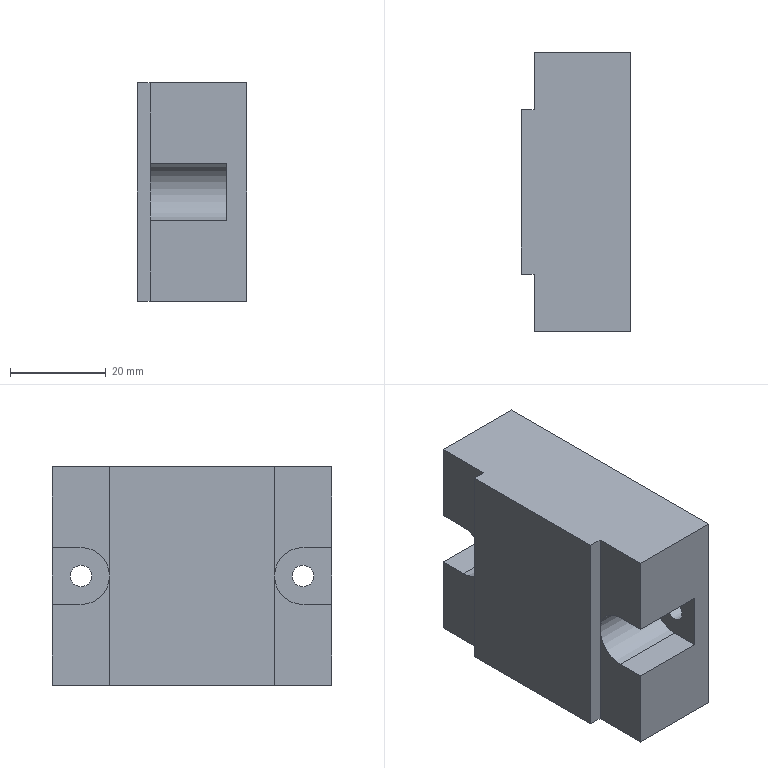Part | NX | features 5003_025_GSR-10L-D32Z 2 | 1 solid | 20 faces | box 22.9 x 58.4 x 45.7 mm | volume 53958 mm3 | plane 16 | cylinder 4 | commonest cylinder face diameters 4.5 x2 11.9 x2
STEP:
#1=CARTESIAN_POINT('',(-263.675,-496.,-115.8));
#2=VERTEX_POINT('',#1);
#3=CARTESIAN_POINT('',(-263.675,-502.,-115.8));
#4=VERTEX_POINT('',#3);
#5=CARTESIAN_POINT('',(-263.675,-502.,-115.8));
#6=DIRECTION('',(0.,-1.,0.));
#7=VECTOR('',#6,1000.);
#8=LINE('',#5,#7);
#9=EDGE_CURVE('',#2,#4,#8,.T.);
#10=ORIENTED_EDGE('',*,*,#9,.F.);
#11=CARTESIAN_POINT('',(-263.675,-496.,-132.7));
#12=VERTEX_POINT('',#11);
#13=CARTESIAN_POINT('',(-263.675,-496.,-87.));
#14=DIRECTION('',(0.,0.,-1.));
#15=VECTOR('',#14,1000.);
#16=LINE('',#13,#15);
#17=EDGE_CURVE('',#2,#12,#16,.T.);
#18=ORIENTED_EDGE('',*,*,#17,.T.);
#19=CARTESIAN_POINT('',(-263.675,-508.,-132.7));
#20=VERTEX_POINT('',#19);
#21=CARTESIAN_POINT('',(-263.675,-496.,-132.7));
#22=DIRECTION('',(0.,-1.,0.));
#23=VECTOR('',#22,1000.);
#24=LINE('',#21,#23);
#25=EDGE_CURVE('',#12,#20,#24,.T.);
#26=ORIENTED_EDGE('',*,*,#25,.T.);
#27=CARTESIAN_POINT('',(-263.675,-508.,-87.));
#28=VERTEX_POINT('',#27);
#29=CARTESIAN_POINT('',(-263.675,-508.,-87.));
#30=DIRECTION('',(0.,0.,-1.));
#31=VECTOR('',#30,1000.);
#32=LINE('',#29,#31);
#33=EDGE_CURVE('',#28,#20,#32,.T.);
#34=ORIENTED_EDGE('',*,*,#33,.F.);
#35=CARTESIAN_POINT('',(-263.675,-496.,-87.));
#36=VERTEX_POINT('',#35);
#37=CARTESIAN_POINT('',(-263.675,-496.,-87.));
#38=DIRECTION('',(0.,1.,0.));
#39=VECTOR('',#38,1000.);
#40=LINE('',#37,#39);
#41=EDGE_CURVE('',#28,#36,#40,.T.);
#42=ORIENTED_EDGE('',*,*,#41,.T.);
#43=CARTESIAN_POINT('',(-263.675,-496.,-103.9));
#44=VERTEX_POINT('',#43);
#45=CARTESIAN_POINT('',(-263.675,-496.,-87.));
#46=DIRECTION('',(0.,0.,-1.));
#47=VECTOR('',#46,1000.);
#48=LINE('',#45,#47);
#49=EDGE_CURVE('',#36,#44,#48,.T.);
#50=ORIENTED_EDGE('',*,*,#49,.T.);
#51=CARTESIAN_POINT('',(-263.675,-502.,-103.9));
#52=VERTEX_POINT('',#51);
#53=CARTESIAN_POINT('',(-263.675,-502.,-103.9));
#54=DIRECTION('',(0.,1.,0.));
#55=VECTOR('',#54,1000.);
#56=LINE('',#53,#55);
#57=EDGE_CURVE('',#52,#44,#56,.T.);
#58=ORIENTED_EDGE('',*,*,#57,.F.);
#59=CARTESIAN_POINT('',(-263.675,-502.,-109.85));
#60=DIRECTION('',(-1.,0.,0.));
#61=DIRECTION('',(0.,0.,-1.));
#62=AXIS2_PLACEMENT_3D('',#59,#60,#61);
#63=CIRCLE('',#62,5.95);
#64=EDGE_CURVE('',#4,#52,#63,.T.);
#65=ORIENTED_EDGE('',*,*,#64,.F.);
#66=EDGE_LOOP('',(#10,#18,#26,#34,#42,#50,#58,#65));
#67=FACE_BOUND('',#66,.T.);
#68=CARTESIAN_POINT('',(-263.675,-496.,-87.));
#69=DIRECTION('',(-1.,0.,0.));
#70=DIRECTION('',(0.,0.,-1.));
#71=AXIS2_PLACEMENT_3D('',#68,#69,#70);
#72=PLANE('',#71);
#73=ADVANCED_FACE('',(#67),#72,.T.);
#74=ORIENTED_EDGE('',*,*,#17,.F.);
#75=CARTESIAN_POINT('',(-247.675,-496.,-115.8));
#76=VERTEX_POINT('',#75);
#77=CARTESIAN_POINT('',(-247.675,-496.,-115.8));
#78=DIRECTION('',(-1.,0.,0.));
#79=VECTOR('',#78,1000.);
#80=LINE('',#77,#79);
#81=EDGE_CURVE('',#76,#2,#80,.T.);
#82=ORIENTED_EDGE('',*,*,#81,.F.);
#83=CARTESIAN_POINT('',(-247.675,-496.,-103.9));
#84=VERTEX_POINT('',#83);
#85=CARTESIAN_POINT('',(-247.675,-496.,-115.8));
#86=DIRECTION('',(0.,0.,-1.));
#87=VECTOR('',#86,1000.);
#88=LINE('',#85,#87);
#89=EDGE_CURVE('',#84,#76,#88,.T.);
#90=ORIENTED_EDGE('',*,*,#89,.F.);
#91=CARTESIAN_POINT('',(-247.675,-496.,-103.9));
#92=DIRECTION('',(-1.,0.,0.));
#93=VECTOR('',#92,1000.);
#94=LINE('',#91,#93);
#95=EDGE_CURVE('',#84,#44,#94,.T.);
#96=ORIENTED_EDGE('',*,*,#95,.T.);
#97=ORIENTED_EDGE('',*,*,#49,.F.);
#98=CARTESIAN_POINT('',(-243.475,-496.,-87.));
#99=VERTEX_POINT('',#98);
#100=CARTESIAN_POINT('',(-263.675,-496.,-87.));
#101=DIRECTION('',(1.,0.,0.));
#102=VECTOR('',#101,1000.);
#103=LINE('',#100,#102);
#104=EDGE_CURVE('',#36,#99,#103,.T.);
#105=ORIENTED_EDGE('',*,*,#104,.T.);
#106=CARTESIAN_POINT('',(-243.475,-496.,-132.7));
#107=VERTEX_POINT('',#106);
#108=CARTESIAN_POINT('',(-243.475,-496.,-87.));
#109=DIRECTION('',(0.,0.,-1.));
#110=VECTOR('',#109,1000.);
#111=LINE('',#108,#110);
#112=EDGE_CURVE('',#99,#107,#111,.T.);
#113=ORIENTED_EDGE('',*,*,#112,.T.);
#114=CARTESIAN_POINT('',(-263.675,-496.,-132.7));
#115=DIRECTION('',(1.,0.,0.));
#116=VECTOR('',#115,1000.);
#117=LINE('',#114,#116);
#118=EDGE_CURVE('',#12,#107,#117,.T.);
#119=ORIENTED_EDGE('',*,*,#118,.F.);
#120=EDGE_LOOP('',(#74,#82,#90,#96,#97,#105,#113,#119));
#121=FACE_BOUND('',#120,.T.);
#122=CARTESIAN_POINT('',(-263.675,-496.,-87.));
#123=DIRECTION('',(0.,-1.,0.));
#124=DIRECTION('',(0.,0.,1.));
#125=AXIS2_PLACEMENT_3D('',#122,#123,#124);
#126=PLANE('',#125);
#127=ADVANCED_FACE('',(#121),#126,.F.);
#128=CARTESIAN_POINT('',(-243.475,-554.4,-132.7));
#129=VERTEX_POINT('',#128);
#130=CARTESIAN_POINT('',(-243.475,-496.,-132.7));
#131=DIRECTION('',(0.,-1.,0.));
#132=VECTOR('',#131,1000.);
#133=LINE('',#130,#132);
#134=EDGE_CURVE('',#107,#129,#133,.T.);
#135=ORIENTED_EDGE('',*,*,#134,.T.);
#136=CARTESIAN_POINT('',(-263.675,-554.4,-132.7));
#137=VERTEX_POINT('',#136);
#138=CARTESIAN_POINT('',(-263.675,-554.4,-132.7));
#139=DIRECTION('',(1.,0.,0.));
#140=VECTOR('',#139,1000.);
#141=LINE('',#138,#140);
#142=EDGE_CURVE('',#137,#129,#141,.T.);
#143=ORIENTED_EDGE('',*,*,#142,.F.);
#144=CARTESIAN_POINT('',(-263.675,-542.4,-132.7));
#145=VERTEX_POINT('',#144);
#146=CARTESIAN_POINT('',(-263.675,-496.,-132.7));
#147=DIRECTION('',(0.,-1.,0.));
#148=VECTOR('',#147,1000.);
#149=LINE('',#146,#148);
#150=EDGE_CURVE('',#145,#137,#149,.T.);
#151=ORIENTED_EDGE('',*,*,#150,.F.);
#152=CARTESIAN_POINT('',(-266.375,-542.4,-132.7));
#153=VERTEX_POINT('',#152);
#154=CARTESIAN_POINT('',(-266.375,-542.4,-132.7));
#155=DIRECTION('',(1.,0.,0.));
#156=VECTOR('',#155,1000.);
#157=LINE('',#154,#156);
#158=EDGE_CURVE('',#153,#145,#157,.T.);
#159=ORIENTED_EDGE('',*,*,#158,.F.);
#160=CARTESIAN_POINT('',(-266.375,-508.,-132.7));
#161=VERTEX_POINT('',#160);
#162=CARTESIAN_POINT('',(-266.375,-508.,-132.7));
#163=DIRECTION('',(0.,-1.,0.));
#164=VECTOR('',#163,1000.);
#165=LINE('',#162,#164);
#166=EDGE_CURVE('',#161,#153,#165,.T.);
#167=ORIENTED_EDGE('',*,*,#166,.F.);
#168=CARTESIAN_POINT('',(-266.375,-508.,-132.7));
#169=DIRECTION('',(1.,0.,0.));
#170=VECTOR('',#169,1000.);
#171=LINE('',#168,#170);
#172=EDGE_CURVE('',#161,#20,#171,.T.);
#173=ORIENTED_EDGE('',*,*,#172,.T.);
#174=ORIENTED_EDGE('',*,*,#25,.F.);
#175=ORIENTED_EDGE('',*,*,#118,.T.);
#176=EDGE_LOOP('',(#135,#143,#151,#159,#167,#173,#174,#175));
#177=FACE_BOUND('',#176,.T.);
#178=CARTESIAN_POINT('',(-263.675,-496.,-132.7));
#179=DIRECTION('',(0.,0.,1.));
#180=DIRECTION('',(0.,1.,0.));
#181=AXIS2_PLACEMENT_3D('',#178,#179,#180);
#182=PLANE('',#181);
#183=ADVANCED_FACE('',(#177),#182,.F.);
#184=CARTESIAN_POINT('',(-263.675,-554.4,-103.9));
#185=VERTEX_POINT('',#184);
#186=CARTESIAN_POINT('',(-263.675,-554.4,-87.));
#187=VERTEX_POINT('',#186);
#188=CARTESIAN_POINT('',(-263.675,-554.4,-87.));
#189=DIRECTION('',(0.,0.,1.));
#190=VECTOR('',#189,1000.);
#191=LINE('',#188,#190);
#192=EDGE_CURVE('',#185,#187,#191,.T.);
#193=ORIENTED_EDGE('',*,*,#192,.F.);
#194=CARTESIAN_POINT('',(-247.675,-554.4,-103.9));
#195=VERTEX_POINT('',#194);
#196=CARTESIAN_POINT('',(-247.675,-554.4,-103.9));
#197=DIRECTION('',(-1.,0.,0.));
#198=VECTOR('',#197,1000.);
#199=LINE('',#196,#198);
#200=EDGE_CURVE('',#195,#185,#199,.T.);
#201=ORIENTED_EDGE('',*,*,#200,.F.);
#202=CARTESIAN_POINT('',(-247.675,-554.4,-115.8));
#203=VERTEX_POINT('',#202);
#204=CARTESIAN_POINT('',(-247.675,-554.4,-115.8));
#205=DIRECTION('',(0.,0.,1.));
#206=VECTOR('',#205,1000.);
#207=LINE('',#204,#206);
#208=EDGE_CURVE('',#203,#195,#207,.T.);
#209=ORIENTED_EDGE('',*,*,#208,.F.);
#210=CARTESIAN_POINT('',(-263.675,-554.4,-115.8));
#211=VERTEX_POINT('',#210);
#212=CARTESIAN_POINT('',(-247.675,-554.4,-115.8));
#213=DIRECTION('',(-1.,0.,0.));
#214=VECTOR('',#213,1000.);
#215=LINE('',#212,#214);
#216=EDGE_CURVE('',#203,#211,#215,.T.);
#217=ORIENTED_EDGE('',*,*,#216,.T.);
#218=CARTESIAN_POINT('',(-263.675,-554.4,-87.));
#219=DIRECTION('',(0.,0.,1.));
#220=VECTOR('',#219,1000.);
#221=LINE('',#218,#220);
#222=EDGE_CURVE('',#137,#211,#221,.T.);
#223=ORIENTED_EDGE('',*,*,#222,.F.);
#224=ORIENTED_EDGE('',*,*,#142,.T.);
#225=CARTESIAN_POINT('',(-243.475,-554.4,-87.));
#226=VERTEX_POINT('',#225);
#227=CARTESIAN_POINT('',(-243.475,-554.4,-87.));
#228=DIRECTION('',(0.,0.,1.));
#229=VECTOR('',#228,1000.);
#230=LINE('',#227,#229);
#231=EDGE_CURVE('',#129,#226,#230,.T.);
#232=ORIENTED_EDGE('',*,*,#231,.T.);
#233=CARTESIAN_POINT('',(-263.675,-554.4,-87.));
#234=DIRECTION('',(1.,0.,0.));
#235=VECTOR('',#234,1000.);
#236=LINE('',#233,#235);
#237=EDGE_CURVE('',#187,#226,#236,.T.);
#238=ORIENTED_EDGE('',*,*,#237,.F.);
#239=EDGE_LOOP('',(#193,#201,#209,#217,#223,#224,#232,#238));
#240=FACE_BOUND('',#239,.T.);
#241=CARTESIAN_POINT('',(-263.675,-554.4,-87.));
#242=DIRECTION('',(0.,1.,0.));
#243=DIRECTION('',(0.,0.,-1.));
#244=AXIS2_PLACEMENT_3D('',#241,#242,#243);
#245=PLANE('',#244);
#246=ADVANCED_FACE('',(#240),#245,.F.);
#247=CARTESIAN_POINT('',(-243.475,-496.,-87.));
#248=DIRECTION('',(0.,1.,0.));
#249=VECTOR('',#248,1000.);
#250=LINE('',#247,#249);
#251=EDGE_CURVE('',#226,#99,#250,.T.);
#252=ORIENTED_EDGE('',*,*,#251,.T.);
#253=ORIENTED_EDGE('',*,*,#104,.F.);
#254=ORIENTED_EDGE('',*,*,#41,.F.);
#255=CARTESIAN_POINT('',(-266.375,-508.,-87.));
#256=VERTEX_POINT('',#255);
#257=CARTESIAN_POINT('',(-266.375,-508.,-87.));
#258=DIRECTION('',(1.,0.,0.));
#259=VECTOR('',#258,1000.);
#260=LINE('',#257,#259);
#261=EDGE_CURVE('',#256,#28,#260,.T.);
#262=ORIENTED_EDGE('',*,*,#261,.F.);
#263=CARTESIAN_POINT('',(-266.375,-542.4,-87.));
#264=VERTEX_POINT('',#263);
#265=CARTESIAN_POINT('',(-266.375,-508.,-87.));
#266=DIRECTION('',(0.,1.,0.));
#267=VECTOR('',#266,1000.);
#268=LINE('',#265,#267);
#269=EDGE_CURVE('',#264,#256,#268,.T.);
#270=ORIENTED_EDGE('',*,*,#269,.F.);
#271=CARTESIAN_POINT('',(-263.675,-542.4,-87.));
#272=VERTEX_POINT('',#271);
#273=CARTESIAN_POINT('',(-266.375,-542.4,-87.));
#274=DIRECTION('',(1.,0.,0.));
#275=VECTOR('',#274,1000.);
#276=LINE('',#273,#275);
#277=EDGE_CURVE('',#264,#272,#276,.T.);
#278=ORIENTED_EDGE('',*,*,#277,.T.);
#279=CARTESIAN_POINT('',(-263.675,-496.,-87.));
#280=DIRECTION('',(0.,1.,0.));
#281=VECTOR('',#280,1000.);
#282=LINE('',#279,#281);
#283=EDGE_CURVE('',#187,#272,#282,.T.);
#284=ORIENTED_EDGE('',*,*,#283,.F.);
#285=ORIENTED_EDGE('',*,*,#237,.T.);
#286=EDGE_LOOP('',(#252,#253,#254,#262,#270,#278,#284,#285));
#287=FACE_BOUND('',#286,.T.);
#288=CARTESIAN_POINT('',(-263.675,-496.,-87.));
#289=DIRECTION('',(0.,0.,-1.));
#290=DIRECTION('',(0.,-1.,0.));
#291=AXIS2_PLACEMENT_3D('',#288,#289,#290);
#292=PLANE('',#291);
#293=ADVANCED_FACE('',(#287),#292,.F.);
#294=CARTESIAN_POINT('',(-263.675,-548.4,-103.9));
#295=VERTEX_POINT('',#294);
#296=CARTESIAN_POINT('',(-263.675,-548.4,-103.9));
#297=DIRECTION('',(0.,1.,0.));
#298=VECTOR('',#297,1000.);
#299=LINE('',#296,#298);
#300=EDGE_CURVE('',#185,#295,#299,.T.);
#301=ORIENTED_EDGE('',*,*,#300,.F.);
#302=ORIENTED_EDGE('',*,*,#192,.T.);
#303=ORIENTED_EDGE('',*,*,#283,.T.);
#304=CARTESIAN_POINT('',(-263.675,-542.4,-87.));
#305=DIRECTION('',(0.,0.,1.));
#306=VECTOR('',#305,1000.);
#307=LINE('',#304,#306);
#308=EDGE_CURVE('',#145,#272,#307,.T.);
#309=ORIENTED_EDGE('',*,*,#308,.F.);
#310=ORIENTED_EDGE('',*,*,#150,.T.);
#311=ORIENTED_EDGE('',*,*,#222,.T.);
#312=CARTESIAN_POINT('',(-263.675,-548.4,-115.8));
#313=VERTEX_POINT('',#312);
#314=CARTESIAN_POINT('',(-263.675,-548.4,-115.8));
#315=DIRECTION('',(0.,-1.,0.));
#316=VECTOR('',#315,1000.);
#317=LINE('',#314,#316);
#318=EDGE_CURVE('',#313,#211,#317,.T.);
#319=ORIENTED_EDGE('',*,*,#318,.F.);
#320=CARTESIAN_POINT('',(-263.675,-548.4,-109.85));
#321=DIRECTION('',(-1.,0.,0.));
#322=DIRECTION('',(0.,0.,1.));
#323=AXIS2_PLACEMENT_3D('',#320,#321,#322);
#324=CIRCLE('',#323,5.95);
#325=EDGE_CURVE('',#295,#313,#324,.T.);
#326=ORIENTED_EDGE('',*,*,#325,.F.);
#327=EDGE_LOOP('',(#301,#302,#303,#309,#310,#311,#319,#326));
#328=FACE_BOUND('',#327,.T.);
#329=CARTESIAN_POINT('',(-263.675,-496.,-87.));
#330=DIRECTION('',(-1.,0.,0.));
#331=DIRECTION('',(0.,0.,-1.));
#332=AXIS2_PLACEMENT_3D('',#329,#330,#331);
#333=PLANE('',#332);
#334=ADVANCED_FACE('',(#328),#333,.T.);
#335=CARTESIAN_POINT('',(-243.475,-502.,-112.1));
#336=VERTEX_POINT('',#335);
#337=CARTESIAN_POINT('',(-243.475,-502.,-109.85));
#338=DIRECTION('',(-1.,0.,0.));
#339=DIRECTION('',(0.,0.,-1.));
#340=AXIS2_PLACEMENT_3D('',#337,#338,#339);
#341=CIRCLE('',#340,2.25);
#342=EDGE_CURVE('',#336,#336,#341,.T.);
#343=ORIENTED_EDGE('',*,*,#342,.T.);
#344=EDGE_LOOP('',(#343));
#345=FACE_BOUND('',#344,.T.);
#346=CARTESIAN_POINT('',(-243.475,-548.4,-112.1));
#347=VERTEX_POINT('',#346);
#348=CARTESIAN_POINT('',(-243.475,-548.4,-109.85));
#349=DIRECTION('',(-1.,0.,0.));
#350=DIRECTION('',(0.,0.,-1.));
#351=AXIS2_PLACEMENT_3D('',#348,#349,#350);
#352=CIRCLE('',#351,2.25);
#353=EDGE_CURVE('',#347,#347,#352,.T.);
#354=ORIENTED_EDGE('',*,*,#353,.T.);
#355=EDGE_LOOP('',(#354));
#356=FACE_BOUND('',#355,.T.);
#357=ORIENTED_EDGE('',*,*,#112,.F.);
#358=ORIENTED_EDGE('',*,*,#251,.F.);
#359=ORIENTED_EDGE('',*,*,#231,.F.);
#360=ORIENTED_EDGE('',*,*,#134,.F.);
#361=EDGE_LOOP('',(#357,#358,#359,#360));
#362=FACE_BOUND('',#361,.T.);
#363=CARTESIAN_POINT('',(-243.475,-496.,-87.));
#364=DIRECTION('',(-1.,0.,0.));
#365=DIRECTION('',(0.,0.,-1.));
#366=AXIS2_PLACEMENT_3D('',#363,#364,#365);
#367=PLANE('',#366);
#368=ADVANCED_FACE('',(#345,#356,#362),#367,.F.);
#369=ORIENTED_EDGE('',*,*,#33,.T.);
#370=ORIENTED_EDGE('',*,*,#172,.F.);
#371=CARTESIAN_POINT('',(-266.375,-508.,-87.));
#372=DIRECTION('',(0.,0.,-1.));
#373=VECTOR('',#372,1000.);
#374=LINE('',#371,#373);
#375=EDGE_CURVE('',#256,#161,#374,.T.);
#376=ORIENTED_EDGE('',*,*,#375,.F.);
#377=ORIENTED_EDGE('',*,*,#261,.T.);
#378=EDGE_LOOP('',(#369,#370,#376,#377));
#379=FACE_BOUND('',#378,.T.);
#380=CARTESIAN_POINT('',(-266.375,-508.,-87.));
#381=DIRECTION('',(0.,-1.,0.));
#382=DIRECTION('',(0.,0.,1.));
#383=AXIS2_PLACEMENT_3D('',#380,#381,#382);
#384=PLANE('',#383);
#385=ADVANCED_FACE('',(#379),#384,.F.);
#386=ORIENTED_EDGE('',*,*,#308,.T.);
#387=ORIENTED_EDGE('',*,*,#277,.F.);
#388=CARTESIAN_POINT('',(-266.375,-542.4,-87.));
#389=DIRECTION('',(0.,0.,1.));
#390=VECTOR('',#389,1000.);
#391=LINE('',#388,#390);
#392=EDGE_CURVE('',#153,#264,#391,.T.);
#393=ORIENTED_EDGE('',*,*,#392,.F.);
#394=ORIENTED_EDGE('',*,*,#158,.T.);
#395=EDGE_LOOP('',(#386,#387,#393,#394));
#396=FACE_BOUND('',#395,.T.);
#397=CARTESIAN_POINT('',(-266.375,-542.4,-87.));
#398=DIRECTION('',(0.,1.,0.));
#399=DIRECTION('',(0.,0.,-1.));
#400=AXIS2_PLACEMENT_3D('',#397,#398,#399);
#401=PLANE('',#400);
#402=ADVANCED_FACE('',(#396),#401,.F.);
#403=ORIENTED_EDGE('',*,*,#375,.T.);
#404=ORIENTED_EDGE('',*,*,#166,.T.);
#405=ORIENTED_EDGE('',*,*,#392,.T.);
#406=ORIENTED_EDGE('',*,*,#269,.T.);
#407=EDGE_LOOP('',(#403,#404,#405,#406));
#408=FACE_BOUND('',#407,.T.);
#409=CARTESIAN_POINT('',(-266.375,-496.,-87.));
#410=DIRECTION('',(-1.,0.,0.));
#411=DIRECTION('',(0.,0.,-1.));
#412=AXIS2_PLACEMENT_3D('',#409,#410,#411);
#413=PLANE('',#412);
#414=ADVANCED_FACE('',(#408),#413,.T.);
#415=ORIENTED_EDGE('',*,*,#325,.T.);
#416=CARTESIAN_POINT('',(-247.675,-548.4,-115.8));
#417=VERTEX_POINT('',#416);
#418=CARTESIAN_POINT('',(-247.675,-548.4,-115.8));
#419=DIRECTION('',(-1.,0.,0.));
#420=VECTOR('',#419,1000.);
#421=LINE('',#418,#420);
#422=EDGE_CURVE('',#417,#313,#421,.T.);
#423=ORIENTED_EDGE('',*,*,#422,.F.);
#424=CARTESIAN_POINT('',(-247.675,-548.4,-103.9));
#425=VERTEX_POINT('',#424);
#426=CARTESIAN_POINT('',(-247.675,-548.4,-109.85));
#427=DIRECTION('',(-1.,0.,0.));
#428=DIRECTION('',(0.,0.,1.));
#429=AXIS2_PLACEMENT_3D('',#426,#427,#428);
#430=CIRCLE('',#429,5.95);
#431=EDGE_CURVE('',#425,#417,#430,.T.);
#432=ORIENTED_EDGE('',*,*,#431,.F.);
#433=CARTESIAN_POINT('',(-247.675,-548.4,-103.9));
#434=DIRECTION('',(-1.,0.,0.));
#435=VECTOR('',#434,1000.);
#436=LINE('',#433,#435);
#437=EDGE_CURVE('',#425,#295,#436,.T.);
#438=ORIENTED_EDGE('',*,*,#437,.T.);
#439=EDGE_LOOP('',(#415,#423,#432,#438));
#440=FACE_BOUND('',#439,.T.);
#441=CARTESIAN_POINT('',(-247.675,-548.4,-109.85));
#442=DIRECTION('',(-1.,0.,0.));
#443=DIRECTION('',(0.,0.,-1.));
#444=AXIS2_PLACEMENT_3D('',#441,#442,#443);
#445=CYLINDRICAL_SURFACE('',#444,5.95);
#446=ADVANCED_FACE('',(#440),#445,.F.);
#447=ORIENTED_EDGE('',*,*,#300,.T.);
#448=ORIENTED_EDGE('',*,*,#437,.F.);
#449=CARTESIAN_POINT('',(-247.675,-548.4,-103.9));
#450=DIRECTION('',(0.,1.,0.));
#451=VECTOR('',#450,1000.);
#452=LINE('',#449,#451);
#453=EDGE_CURVE('',#195,#425,#452,.T.);
#454=ORIENTED_EDGE('',*,*,#453,.F.);
#455=ORIENTED_EDGE('',*,*,#200,.T.);
#456=EDGE_LOOP('',(#447,#448,#454,#455));
#457=FACE_BOUND('',#456,.T.);
#458=CARTESIAN_POINT('',(-247.675,-548.4,-103.9));
#459=DIRECTION('',(0.,0.,1.));
#460=DIRECTION('',(0.,1.,0.));
#461=AXIS2_PLACEMENT_3D('',#458,#459,#460);
#462=PLANE('',#461);
#463=ADVANCED_FACE('',(#457),#462,.F.);
#464=ORIENTED_EDGE('',*,*,#318,.T.);
#465=ORIENTED_EDGE('',*,*,#216,.F.);
#466=CARTESIAN_POINT('',(-247.675,-548.4,-115.8));
#467=DIRECTION('',(0.,-1.,0.));
#468=VECTOR('',#467,1000.);
#469=LINE('',#466,#468);
#470=EDGE_CURVE('',#417,#203,#469,.T.);
#471=ORIENTED_EDGE('',*,*,#470,.F.);
#472=ORIENTED_EDGE('',*,*,#422,.T.);
#473=EDGE_LOOP('',(#464,#465,#471,#472));
#474=FACE_BOUND('',#473,.T.);
#475=CARTESIAN_POINT('',(-247.675,-548.4,-115.8));
#476=DIRECTION('',(0.,0.,-1.));
#477=DIRECTION('',(0.,-1.,0.));
#478=AXIS2_PLACEMENT_3D('',#475,#476,#477);
#479=PLANE('',#478);
#480=ADVANCED_FACE('',(#474),#479,.F.);
#481=CARTESIAN_POINT('',(-247.675,-548.4,-112.1));
#482=VERTEX_POINT('',#481);
#483=CARTESIAN_POINT('',(-247.675,-548.4,-109.85));
#484=DIRECTION('',(-1.,0.,0.));
#485=DIRECTION('',(0.,0.,-1.));
#486=AXIS2_PLACEMENT_3D('',#483,#484,#485);
#487=CIRCLE('',#486,2.25);
#488=EDGE_CURVE('',#482,#482,#487,.T.);
#489=ORIENTED_EDGE('',*,*,#488,.F.);
#490=EDGE_LOOP('',(#489));
#491=FACE_BOUND('',#490,.T.);
#492=ORIENTED_EDGE('',*,*,#431,.T.);
#493=ORIENTED_EDGE('',*,*,#470,.T.);
#494=ORIENTED_EDGE('',*,*,#208,.T.);
#495=ORIENTED_EDGE('',*,*,#453,.T.);
#496=EDGE_LOOP('',(#492,#493,#494,#495));
#497=FACE_BOUND('',#496,.T.);
#498=CARTESIAN_POINT('',(-247.675,-548.4,-109.85));
#499=DIRECTION('',(1.,0.,0.));
#500=DIRECTION('',(0.,0.,1.));
#501=AXIS2_PLACEMENT_3D('',#498,#499,#500);
#502=PLANE('',#501);
#503=ADVANCED_FACE('',(#491,#497),#502,.F.);
#504=ORIENTED_EDGE('',*,*,#64,.T.);
#505=CARTESIAN_POINT('',(-247.675,-502.,-103.9));
#506=VERTEX_POINT('',#505);
#507=CARTESIAN_POINT('',(-247.675,-502.,-103.9));
#508=DIRECTION('',(-1.,0.,0.));
#509=VECTOR('',#508,1000.);
#510=LINE('',#507,#509);
#511=EDGE_CURVE('',#506,#52,#510,.T.);
#512=ORIENTED_EDGE('',*,*,#511,.F.);
#513=CARTESIAN_POINT('',(-247.675,-502.,-115.8));
#514=VERTEX_POINT('',#513);
#515=CARTESIAN_POINT('',(-247.675,-502.,-109.85));
#516=DIRECTION('',(-1.,0.,0.));
#517=DIRECTION('',(0.,0.,-1.));
#518=AXIS2_PLACEMENT_3D('',#515,#516,#517);
#519=CIRCLE('',#518,5.95);
#520=EDGE_CURVE('',#514,#506,#519,.T.);
#521=ORIENTED_EDGE('',*,*,#520,.F.);
#522=CARTESIAN_POINT('',(-247.675,-502.,-115.8));
#523=DIRECTION('',(-1.,0.,0.));
#524=VECTOR('',#523,1000.);
#525=LINE('',#522,#524);
#526=EDGE_CURVE('',#514,#4,#525,.T.);
#527=ORIENTED_EDGE('',*,*,#526,.T.);
#528=EDGE_LOOP('',(#504,#512,#521,#527));
#529=FACE_BOUND('',#528,.T.);
#530=CARTESIAN_POINT('',(-247.675,-502.,-109.85));
#531=DIRECTION('',(-1.,0.,0.));
#532=DIRECTION('',(0.,0.,-1.));
#533=AXIS2_PLACEMENT_3D('',#530,#531,#532);
#534=CYLINDRICAL_SURFACE('',#533,5.95);
#535=ADVANCED_FACE('',(#529),#534,.F.);
#536=ORIENTED_EDGE('',*,*,#9,.T.);
#537=ORIENTED_EDGE('',*,*,#526,.F.);
#538=CARTESIAN_POINT('',(-247.675,-502.,-115.8));
#539=DIRECTION('',(0.,-1.,0.));
#540=VECTOR('',#539,1000.);
#541=LINE('',#538,#540);
#542=EDGE_CURVE('',#76,#514,#541,.T.);
#543=ORIENTED_EDGE('',*,*,#542,.F.);
#544=ORIENTED_EDGE('',*,*,#81,.T.);
#545=EDGE_LOOP('',(#536,#537,#543,#544));
#546=FACE_BOUND('',#545,.T.);
#547=CARTESIAN_POINT('',(-247.675,-502.,-115.8));
#548=DIRECTION('',(0.,0.,-1.));
#549=DIRECTION('',(0.,-1.,0.));
#550=AXIS2_PLACEMENT_3D('',#547,#548,#549);
#551=PLANE('',#550);
#552=ADVANCED_FACE('',(#546),#551,.F.);
#553=ORIENTED_EDGE('',*,*,#57,.T.);
#554=ORIENTED_EDGE('',*,*,#95,.F.);
#555=CARTESIAN_POINT('',(-247.675,-502.,-103.9));
#556=DIRECTION('',(0.,1.,0.));
#557=VECTOR('',#556,1000.);
#558=LINE('',#555,#557);
#559=EDGE_CURVE('',#506,#84,#558,.T.);
#560=ORIENTED_EDGE('',*,*,#559,.F.);
#561=ORIENTED_EDGE('',*,*,#511,.T.);
#562=EDGE_LOOP('',(#553,#554,#560,#561));
#563=FACE_BOUND('',#562,.T.);
#564=CARTESIAN_POINT('',(-247.675,-502.,-103.9));
#565=DIRECTION('',(0.,0.,1.));
#566=DIRECTION('',(0.,1.,0.));
#567=AXIS2_PLACEMENT_3D('',#564,#565,#566);
#568=PLANE('',#567);
#569=ADVANCED_FACE('',(#563),#568,.F.);
#570=CARTESIAN_POINT('',(-247.675,-502.,-112.1));
#571=VERTEX_POINT('',#570);
#572=CARTESIAN_POINT('',(-247.675,-502.,-109.85));
#573=DIRECTION('',(-1.,0.,0.));
#574=DIRECTION('',(0.,0.,-1.));
#575=AXIS2_PLACEMENT_3D('',#572,#573,#574);
#576=CIRCLE('',#575,2.25);
#577=EDGE_CURVE('',#571,#571,#576,.T.);
#578=ORIENTED_EDGE('',*,*,#577,.F.);
#579=EDGE_LOOP('',(#578));
#580=FACE_BOUND('',#579,.T.);
#581=ORIENTED_EDGE('',*,*,#520,.T.);
#582=ORIENTED_EDGE('',*,*,#559,.T.);
#583=ORIENTED_EDGE('',*,*,#89,.T.);
#584=ORIENTED_EDGE('',*,*,#542,.T.);
#585=EDGE_LOOP('',(#581,#582,#583,#584));
#586=FACE_BOUND('',#585,.T.);
#587=CARTESIAN_POINT('',(-247.675,-502.,-109.85));
#588=DIRECTION('',(-1.,0.,0.));
#589=DIRECTION('',(0.,0.,-1.));
#590=AXIS2_PLACEMENT_3D('',#587,#588,#589);
#591=PLANE('',#590);
#592=ADVANCED_FACE('',(#580,#586),#591,.T.);
#593=ORIENTED_EDGE('',*,*,#342,.F.);
#594=EDGE_LOOP('',(#593));
#595=FACE_BOUND('',#594,.T.);
#596=ORIENTED_EDGE('',*,*,#577,.T.);
#597=EDGE_LOOP('',(#596));
#598=FACE_BOUND('',#597,.T.);
#599=CARTESIAN_POINT('',(-243.475,-502.,-109.85));
#600=DIRECTION('',(-1.,0.,0.));
#601=DIRECTION('',(0.,0.,-1.));
#602=AXIS2_PLACEMENT_3D('',#599,#600,#601);
#603=CYLINDRICAL_SURFACE('',#602,2.25);
#604=ADVANCED_FACE('',(#595,#598),#603,.F.);
#605=ORIENTED_EDGE('',*,*,#353,.F.);
#606=EDGE_LOOP('',(#605));
#607=FACE_BOUND('',#606,.T.);
#608=ORIENTED_EDGE('',*,*,#488,.T.);
#609=EDGE_LOOP('',(#608));
#610=FACE_BOUND('',#609,.T.);
#611=CARTESIAN_POINT('',(-243.475,-548.4,-109.85));
#612=DIRECTION('',(-1.,0.,0.));
#613=DIRECTION('',(0.,0.,-1.));
#614=AXIS2_PLACEMENT_3D('',#611,#612,#613);
#615=CYLINDRICAL_SURFACE('',#614,2.25);
#616=ADVANCED_FACE('',(#607,#610),#615,.F.);
#617=CLOSED_SHELL('',(#73,#127,#183,#246,#293,#334,#368,#385,#402,#414,#446,#463,#480,#503,#535,#552,#569,#592,#604,#616));
#618=MANIFOLD_SOLID_BREP('',#617);
#619=(LENGTH_UNIT()NAMED_UNIT(*)SI_UNIT(.MILLI.,.METRE.));
#620=UNCERTAINTY_MEASURE_WITH_UNIT(LENGTH_MEASURE(0.00001),#619,'','');
#621=(NAMED_UNIT(*)PLANE_ANGLE_UNIT()SI_UNIT($,.RADIAN.));
#622=(NAMED_UNIT(*)SI_UNIT($,.STERADIAN.)SOLID_ANGLE_UNIT());
#623=(GEOMETRIC_REPRESENTATION_CONTEXT(3)GLOBAL_UNCERTAINTY_ASSIGNED_CONTEXT((#620))GLOBAL_UNIT_ASSIGNED_CONTEXT((#619,#621,#622))REPRESENTATION_CONTEXT('',''));
#624=ADVANCED_BREP_SHAPE_REPRESENTATION('',(#618),#623);